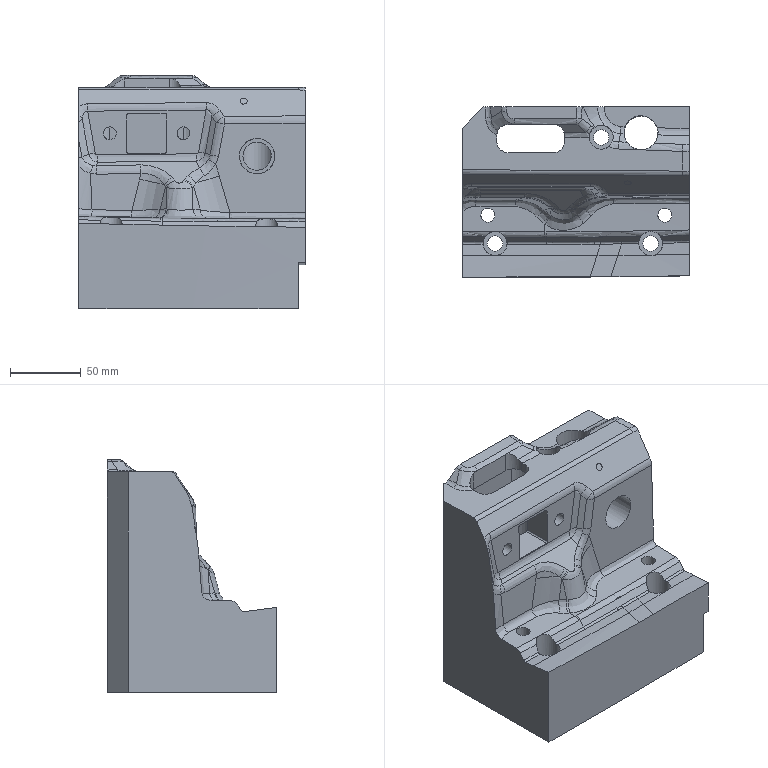Part | NX | features solid 2 | 1 solid | 160 faces | box 160 x 120.169 x 164.792 mm | volume 1580724 mm3 | spline 112 | cylinder 25 | plane 23 | commonest cylinder face diameters 2.1 x4 16 x4 18 x4 11 x3 17 x3 9.1 x2